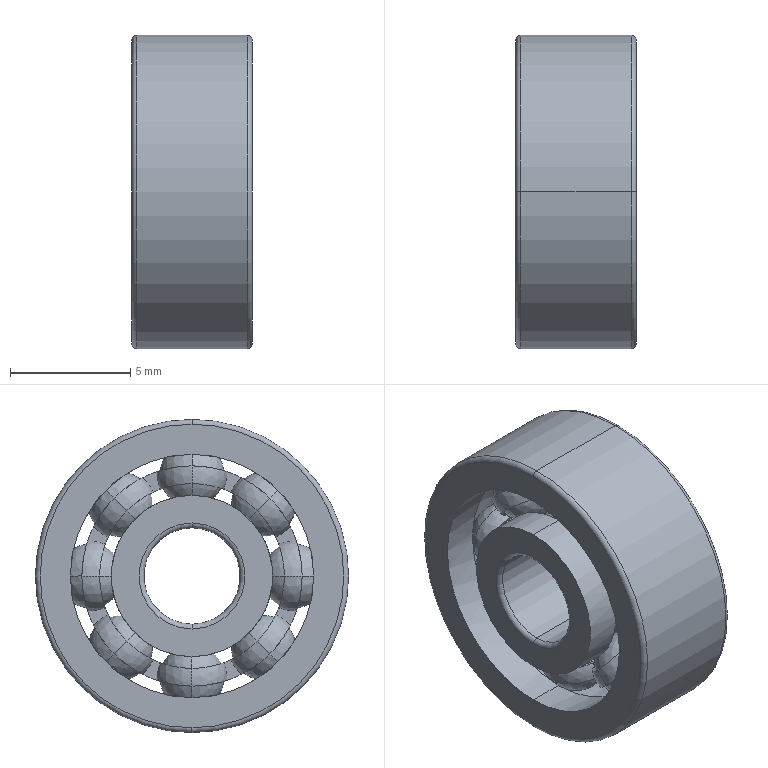Part | NX | features BREP 1 | 1 solid | 132 faces | box 5 x 13 x 13 mm | volume 428.524 mm3 | sphere 64 | torus 32 | plane 20 | cylinder 16 | commonest cylinder face diameters 6.7 x4 10.1 x4 4 x2 7.663 x2 9.137 x2 13 x2